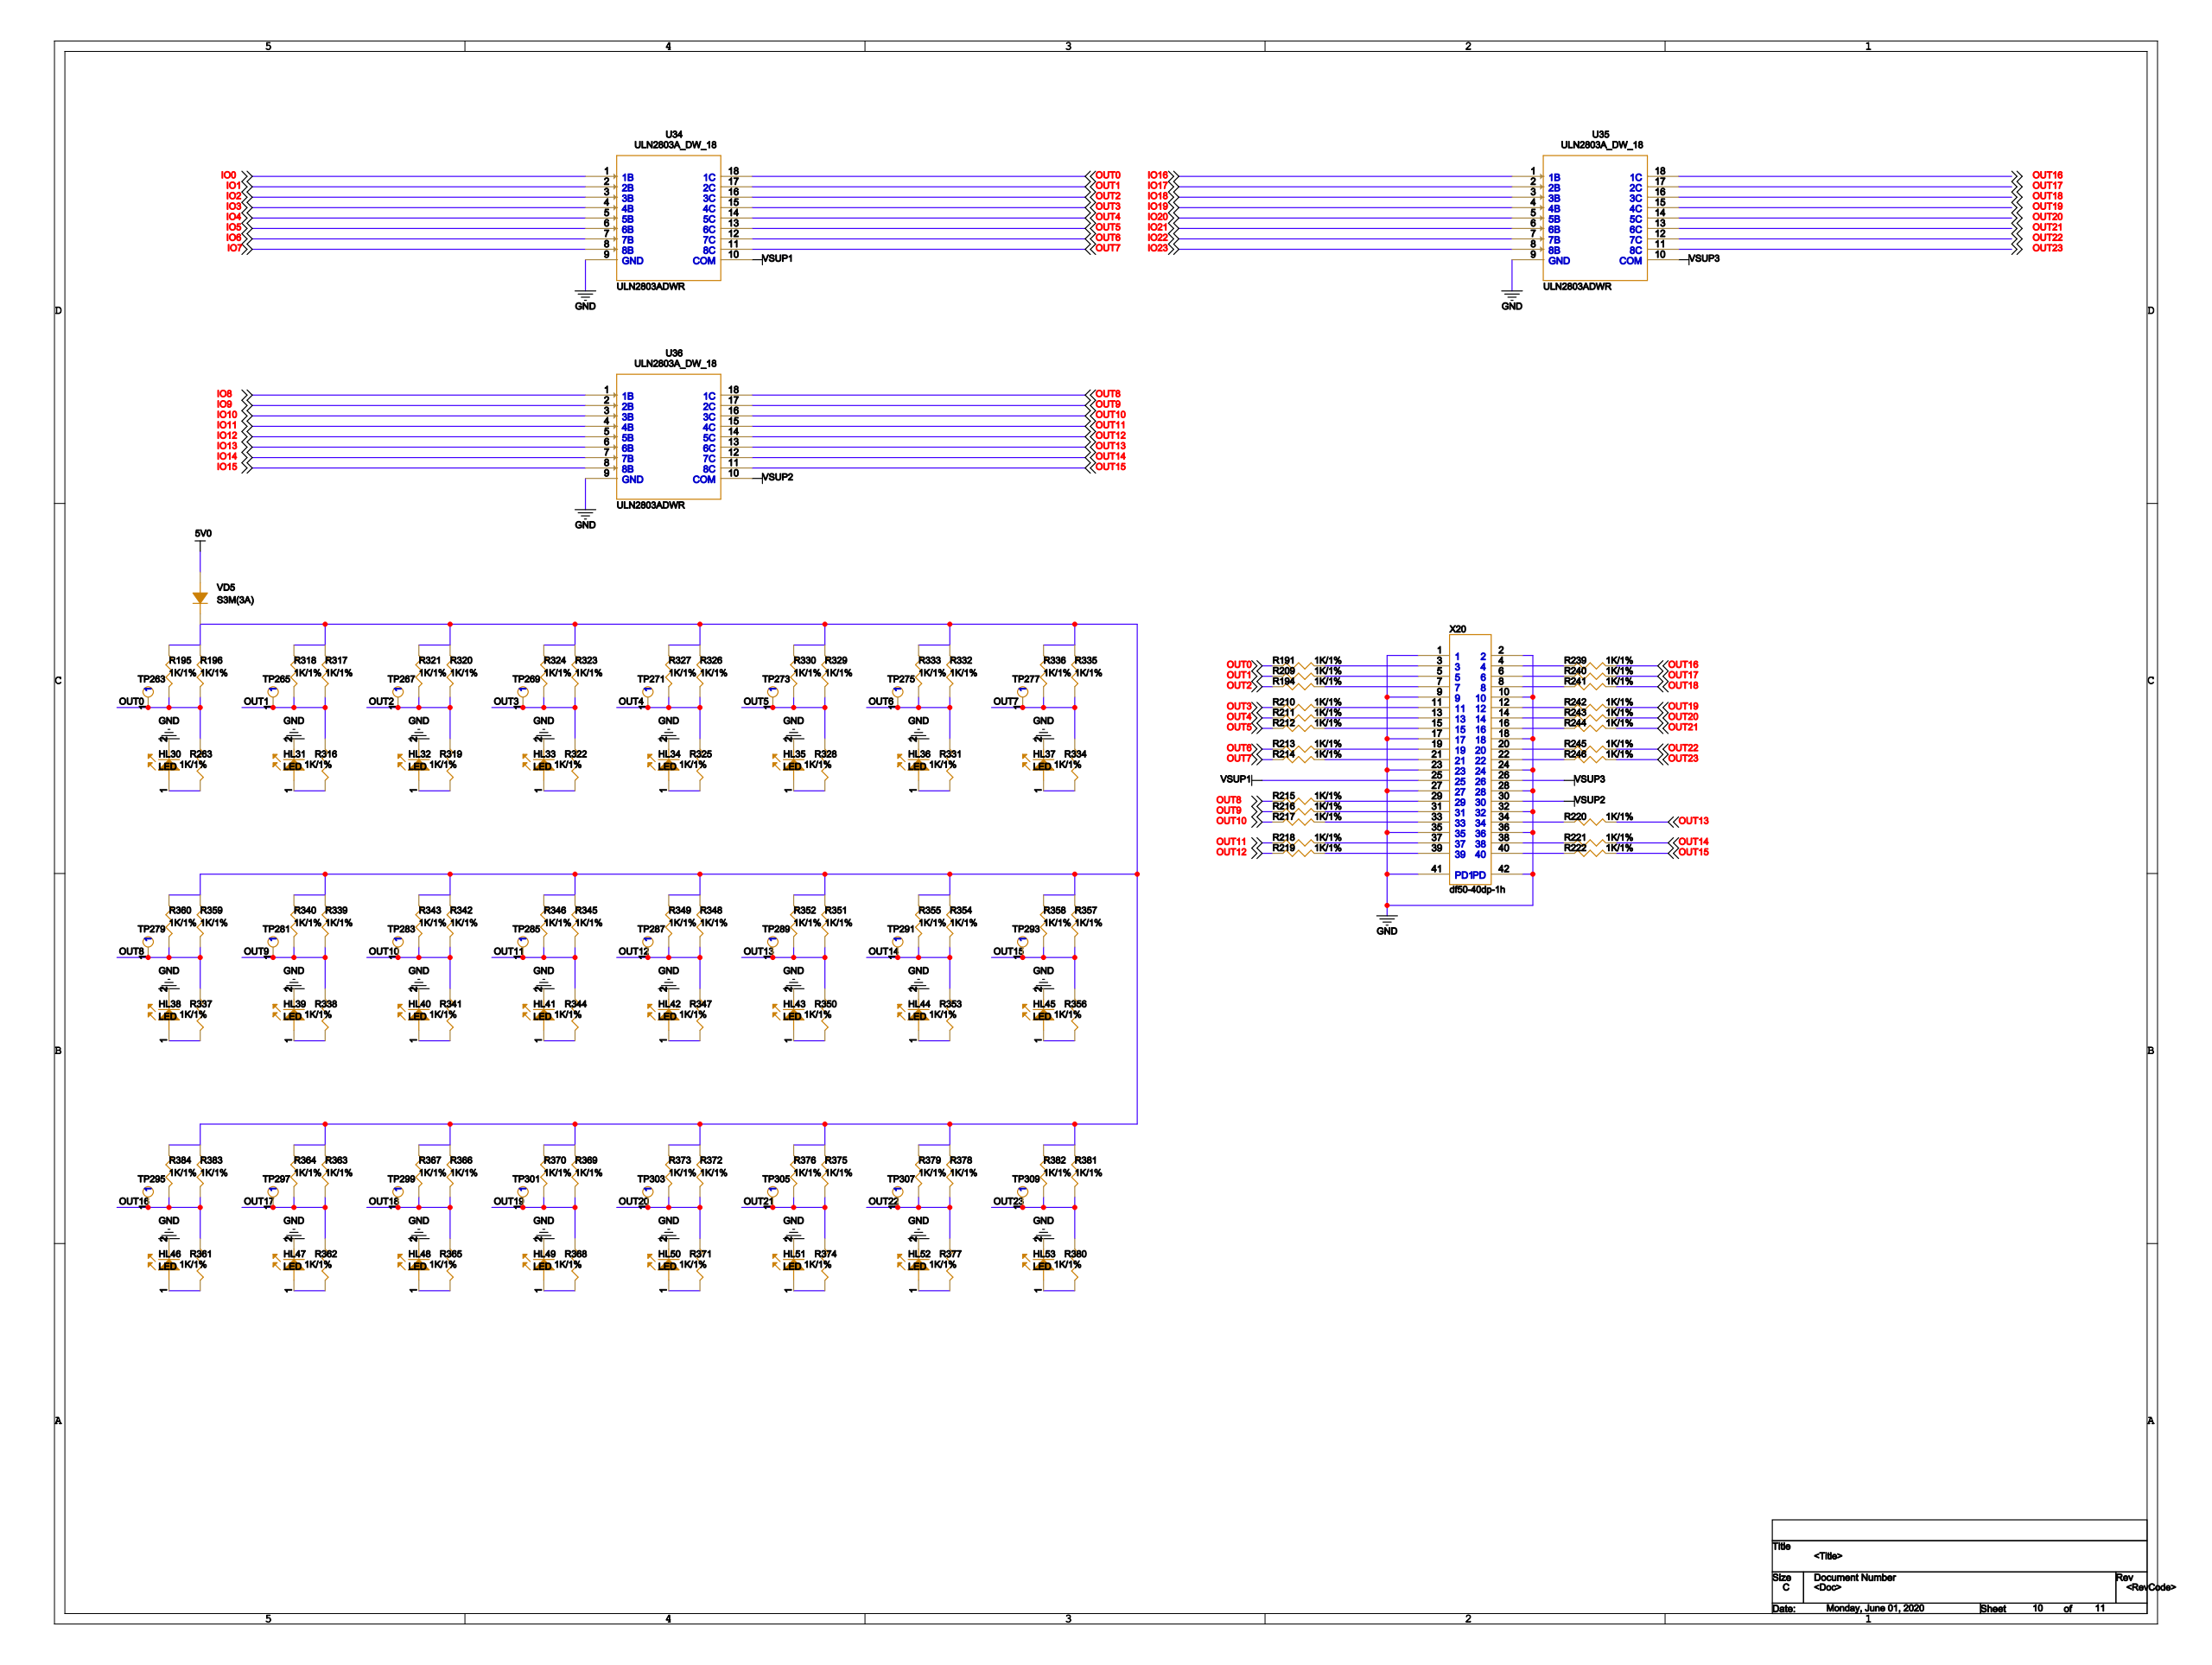Circuit board | Cadence Allegro | 792 parts | 400 nets | one sheet of the schematic
Parts on this sheet (reference | value | footprint):
HL30 | LED | LED0603
HL31 | LED | LED0603
HL32 | LED | LED0603
HL33 | LED | LED0603
HL34 | LED | LED0603
HL35 | LED | LED0603
HL36 | LED | LED0603
HL37 | LED | LED0603
HL38 | LED | LED0603
HL39 | LED | LED0603
HL40 | LED | LED0603
HL41 | LED | LED0603
HL42 | LED | LED0603
HL43 | LED | LED0603
HL44 | LED | LED0603
HL45 | LED | LED0603
HL46 | LED | LED0603
HL47 | LED | LED0603
HL48 | LED | LED0603
HL49 | LED | LED0603
HL50 | LED | LED0603
HL51 | LED | LED0603
HL52 | LED | LED0603
HL53 | LED | LED0603
R191 | 1K/1% | R0603
R194 | 1K/1% | R0603
R195 | 1K/1% | R0603
R196 | 1K/1% | R0603
R209 | 1K/1% | R0603
R210 | 1K/1% | R0603
R211 | 1K/1% | R0603
R212 | 1K/1% | R0603
R213 | 1K/1% | R0603
R214 | 1K/1% | R0603
R215 | 1K/1% | R0603
R216 | 1K/1% | R0603
R217 | 1K/1% | R0603
R218 | 1K/1% | R0603
R219 | 1K/1% | R0603
R220 | 1K/1% | R0603
R221 | 1K/1% | R0603
R222 | 1K/1% | R0603
R239 | 1K/1% | R0603
R240 | 1K/1% | R0603
R241 | 1K/1% | R0603
R242 | 1K/1% | R0603
R243 | 1K/1% | R0603
R244 | 1K/1% | R0603
R245 | 1K/1% | R0603
R246 | 1K/1% | R0603
R263 | 1K/1% | R0603
R316 | 1K/1% | R0603
R317 | 1K/1% | R0603
R318 | 1K/1% | R0603
R319 | 1K/1% | R0603
R320 | 1K/1% | R0603
R321 | 1K/1% | R0603
R322 | 1K/1% | R0603
R323 | 1K/1% | R0603
R324 | 1K/1% | R0603
R325 | 1K/1% | R0603
R326 | 1K/1% | R0603
R327 | 1K/1% | R0603
R328 | 1K/1% | R0603
R329 | 1K/1% | R0603
R330 | 1K/1% | R0603
R331 | 1K/1% | R0603
R332 | 1K/1% | R0603
R333 | 1K/1% | R0603
R334 | 1K/1% | R0603
R335 | 1K/1% | R0603
R336 | 1K/1% | R0603
R337 | 1K/1% | R0603
R338 | 1K/1% | R0603
R339 | 1K/1% | R0603
R340 | 1K/1% | R0603
R341 | 1K/1% | R0603
R342 | 1K/1% | R0603
R343 | 1K/1% | R0603
R344 | 1K/1% | R0603
R345 | 1K/1% | R0603
R346 | 1K/1% | R0603
R347 | 1K/1% | R0603
R348 | 1K/1% | R0603
R349 | 1K/1% | R0603
R350 | 1K/1% | R0603
R351 | 1K/1% | R0603
R352 | 1K/1% | R0603
R353 | 1K/1% | R0603
R354 | 1K/1% | R0603
R355 | 1K/1% | R0603
R356 | 1K/1% | R0603
R357 | 1K/1% | R0603
R358 | 1K/1% | R0603
R359 | 1K/1% | R0603
R360 | 1K/1% | R0603
R361 | 1K/1% | R0603
R362 | 1K/1% | R0603
R363 | 1K/1% | R0603
R364 | 1K/1% | R0603
R365 | 1K/1% | R0603
R366 | 1K/1% | R0603
R367 | 1K/1% | R0603
R368 | 1K/1% | R0603
R369 | 1K/1% | R0603
R370 | 1K/1% | R0603
R371 | 1K/1% | R0603
R372 | 1K/1% | R0603
R373 | 1K/1% | R0603
R374 | 1K/1% | R0603
R375 | 1K/1% | R0603
R376 | 1K/1% | R0603
R377 | 1K/1% | R0603
R378 | 1K/1% | R0603
R379 | 1K/1% | R0603
R380 | 1K/1% | R0603
R381 | 1K/1% | R0603
R382 | 1K/1% | R0603
R383 | 1K/1% | R0603
R384 | 1K/1% | R0603
TP263 | TESTPOINT | TESTPOINT-33MIL
TP265 | TESTPOINT | TESTPOINT-33MIL
TP267 | TESTPOINT | TESTPOINT-33MIL
TP269 | TESTPOINT | TESTPOINT-33MIL
TP271 | TESTPOINT | TESTPOINT-33MIL
TP273 | TESTPOINT | TESTPOINT-33MIL
TP275 | TESTPOINT | TESTPOINT-33MIL
TP277 | TESTPOINT | TESTPOINT-33MIL
TP279 | TESTPOINT | TESTPOINT-33MIL
TP281 | TESTPOINT | TESTPOINT-33MIL
TP283 | TESTPOINT | TESTPOINT-33MIL
TP285 | TESTPOINT | TESTPOINT-33MIL
TP287 | TESTPOINT | TESTPOINT-33MIL
TP289 | TESTPOINT | TESTPOINT-33MIL
TP291 | TESTPOINT | TESTPOINT-33MIL
TP293 | TESTPOINT | TESTPOINT-33MIL
TP295 | TESTPOINT | TESTPOINT-33MIL
TP297 | TESTPOINT | TESTPOINT-33MIL
TP299 | TESTPOINT | TESTPOINT-33MIL
TP301 | TESTPOINT | TESTPOINT-33MIL
TP303 | TESTPOINT | TESTPOINT-33MIL
TP305 | TESTPOINT | TESTPOINT-33MIL
TP307 | TESTPOINT | TESTPOINT-33MIL
TP309 | TESTPOINT | TESTPOINT-33MIL
U34 | ULN2803ADWR | SOIC18W
U35 | ULN2803ADWR | SOIC18W
U36 | ULN2803ADWR | SOIC18W
VD5 | S3M(3A) | DIODE_SMA
X20 | df50-40dp-1h | DF50-40DP-1H
Nets of these parts (net: part-pin ...):
GND: HL30-2 HL31-2 HL32-2 HL33-2 HL34-2 HL35-2 HL36-2 HL37-2 HL38-2 HL39-2 HL40-2 HL41-2 HL42-2 HL43-2 HL44-2 HL45-2 HL46-2 HL47-2 HL48-2 HL49-2 HL50-2 HL51-2 HL52-2 HL53-2 U34-9 U35-9 U36-9 X20-1 X20-2 X20-9 X20-10 X20-17 X20-18 X20-23 X20-24 X20-27 X20-28 X20-32 X20-35 X20-36 X20-41 X20-42
N8013113: R210-2 X20-11
N8024737: R242-1 X20-12
N8013117: R211-2 X20-13
N8024735: R243-1 X20-14
N8013121: R212-2 X20-15
N8024733: R244-1 X20-16
N8013125: R213-2 X20-19
N8024731: R245-1 X20-20
N8013129: R214-2 X20-21
N8024729: R246-1 X20-22
VSUP1: U34-10 X20-25
VSUP3: U35-10 X20-26
N8012653: R215-2 X20-29
N8013101: R191-2 X20-3
VSUP2: U36-10 X20-30
N8012657: R216-2 X20-31
N8012661: R217-2 X20-33
N8014428: R220-1 X20-34
N8012665: R218-2 X20-37
N8014432: R221-1 X20-38
N8012669: R219-2 X20-39
N8024743: R239-1 X20-4
N8014430: R222-1 X20-40
N8013105: R209-2 X20-5
N8024741: R240-1 X20-6
N8013109: R194-2 X20-7
N8024739: R241-1 X20-8
OUT1: R209-1 R316-1 R317-2 R318-2 TP265-1 U34-17
N8103771: HL31-1 R316-2
N7907697: R195-1 R196-1 R317-1 R318-1 R320-1 R321-1 R323-1 R324-1 R326-1 R327-1 R329-1 R330-1 R332-1 R333-1 R335-1 R336-1 R339-1 R340-1 R342-1 R343-1 R345-1 R346-1 R348-1 R349-1 R351-1 R352-1 R354-1 R355-1 R357-1 R358-1 R359-1 R360-1 R363-1 R364-1 R366-1 R367-1 R369-1 R370-1 R372-1 R373-1 R375-1 R376-1 R378-1 R379-1 R381-1 R382-1 R383-1 R384-1 VD5-2
OUT2: R194-1 R319-1 R320-2 R321-2 TP267-1 U34-16
N8104165: HL32-1 R319-2
OUT3: R210-1 R322-1 R323-2 R324-2 TP269-1 U34-15
N8104572: HL33-1 R322-2
OUT4: R211-1 R325-1 R326-2 R327-2 TP271-1 U34-14
N8104992: HL34-1 R325-2
OUT5: R212-1 R328-1 R329-2 R330-2 TP273-1 U34-13
N8105424: HL35-1 R328-2
OUT6: R213-1 R331-1 R332-2 R333-2 TP275-1 U34-12
N8105866: HL36-1 R331-2
OUT7: R214-1 R334-1 R335-2 R336-2 TP277-1 U34-11
N8106320: HL37-1 R334-2
OUT8: R215-1 R337-1 R359-2 R360-2 TP279-1 U36-18
N8115416: HL38-1 R337-2
OUT9: R216-1 R338-1 R339-2 R340-2 TP281-1 U36-17
N8115490: HL39-1 R338-2
OUT10: R217-1 R341-1 R342-2 R343-2 TP283-1 U36-16
N8115632: HL40-1 R341-2
OUT11: R218-1 R344-1 R345-2 R346-2 TP285-1 U36-15
N8115760: HL41-1 R344-2
OUT12: R219-1 R347-1 R348-2 R349-2 TP287-1 U36-14
N8115900: HL42-1 R347-2
OUT13: R220-2 R350-1 R351-2 R352-2 TP289-1 U36-13
N8116034: HL43-1 R350-2
OUT14: R221-2 R353-1 R354-2 R355-2 TP291-1 U36-12
N8116162: HL44-1 R353-2
OUT15: R222-2 R356-1 R357-2 R358-2 TP293-1 U36-11
N8116302: HL45-1 R356-2
OUT16: R239-2 R361-1 R383-2 R384-2 TP295-1 U35-18
N8117662: HL46-1 R361-2
OUT17: R240-2 R362-1 R363-2 R364-2 TP297-1 U35-17
N8117736: HL47-1 R362-2
OUT18: R241-2 R365-1 R366-2 R367-2 TP299-1 U35-16
N8117878: HL48-1 R365-2
OUT19: R242-2 R368-1 R369-2 R370-2 TP301-1 U35-15
N8118006: HL49-1 R368-2
OUT20: R243-2 R371-1 R372-2 R373-2 TP303-1 U35-14
N8118146: HL50-1 R371-2
OUT21: R244-2 R374-1 R375-2 R376-2 TP305-1 U35-13
N8118280: HL51-1 R374-2
OUT22: R245-2 R377-1 R378-2 R379-2 TP307-1 U35-12
N8118408: HL52-1 R377-2
OUT23: R246-2 R380-1 R381-2 R382-2 TP309-1 U35-11
N8118548: HL53-1 R380-2
OUT0: R191-1 R195-2 R196-2 R263-1 TP263-1 U34-18
N8090309: HL30-1 R263-2
IO0: U34-1
IO1: U34-2
IO2: U34-3
IO3: U34-4
IO4: U34-5
IO5: U34-6
IO6: U34-7
IO7: U34-8
IO16: U35-1
IO17: U35-2
IO18: U35-3
IO19: U35-4
IO20: U35-5
IO21: U35-6
IO22: U35-7
IO23: U35-8
IO8: U36-1
IO9: U36-2
IO10: U36-3
IO11: U36-4
IO12: U36-5
IO13: U36-6
IO14: U36-7
IO15: U36-8
5V0: VD5-1